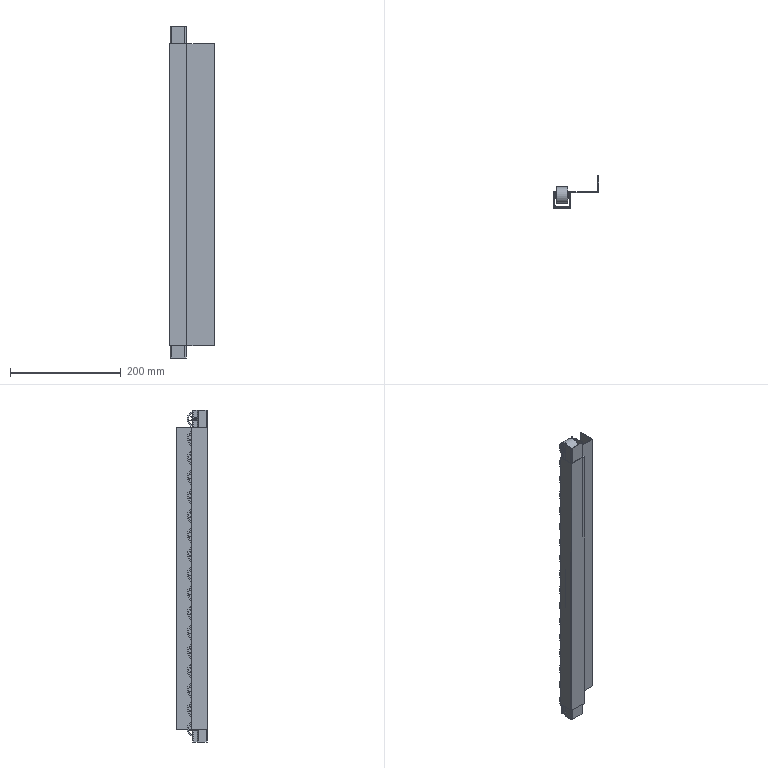Part | STEP file | RIEL CABINA | 35 solids | 984 faces | box 81.4 x 57.7 x 600 mm | volume 321427 mm3 | cylinder 458 | plane 390 | spline 136 | commonest cylinder face diameters 10 x136 25 x136 4 x102 5 x34 30 x34 1.473 x8